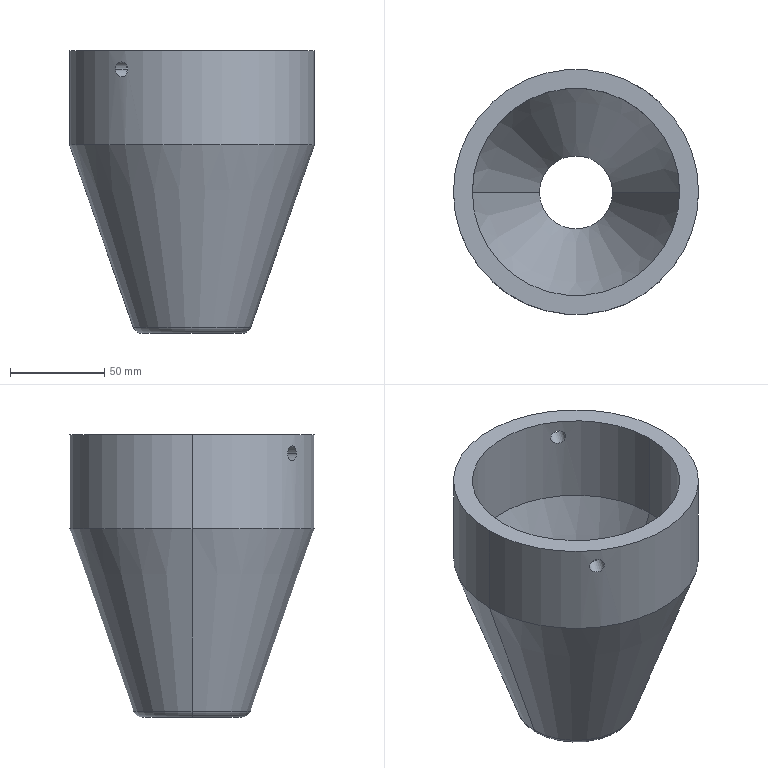Part | SolidWorks | features HoleWzd 2, 3DProfileFeature 1, Fillet 1, Revolution 1 | 1 solid | 16 faces | box 130 x 130 x 150 mm | volume 468175 mm3 | cylinder 8 | cone 4 | torus 2 | plane 2 | commonest cylinder face diameters 8 x4 110 x2 130 x2
STEP:
#1=CARTESIAN_POINT('',(552.403,234.744,-1661.65));
#2=VERTEX_POINT('',#1);
#3=CARTESIAN_POINT('',(490.059,234.744,-1661.65));
#4=VERTEX_POINT('',#3);
#5=CARTESIAN_POINT('',(521.231,234.744,-1661.65));
#6=DIRECTION('',(0.,0.,1.));
#7=DIRECTION('',(-1.,0.,0.));
#8=AXIS2_PLACEMENT_3D('',#5,#6,#7);
#9=CIRCLE('',#8,31.172);
#10=EDGE_CURVE('',#2,#4,#9,.T.);
#11=ORIENTED_EDGE('',*,*,#10,.F.);
#12=CARTESIAN_POINT('',(547.683,234.744,-1664.998));
#13=VERTEX_POINT('',#12);
#14=CARTESIAN_POINT('',(547.683,234.744,-1659.998));
#15=DIRECTION('',(0.,1.,0.));
#16=DIRECTION('',(-1.,0.,0.));
#17=AXIS2_PLACEMENT_3D('',#14,#15,#16);
#18=CIRCLE('',#17,5.);
#19=EDGE_CURVE('',#2,#13,#18,.T.);
#20=ORIENTED_EDGE('',*,*,#19,.T.);
#21=CARTESIAN_POINT('',(494.778,234.744,-1664.998));
#22=VERTEX_POINT('',#21);
#23=CARTESIAN_POINT('',(521.231,234.744,-1664.998));
#24=DIRECTION('',(0.,0.,-1.));
#25=DIRECTION('',(-1.,0.,0.));
#26=AXIS2_PLACEMENT_3D('',#23,#24,#25);
#27=CIRCLE('',#26,26.453);
#28=EDGE_CURVE('',#22,#13,#27,.T.);
#29=ORIENTED_EDGE('',*,*,#28,.F.);
#30=CARTESIAN_POINT('',(494.778,234.744,-1659.998));
#31=DIRECTION('',(0.,-1.,0.));
#32=DIRECTION('',(0.,0.,-1.));
#33=AXIS2_PLACEMENT_3D('',#30,#31,#32);
#34=CIRCLE('',#33,5.);
#35=EDGE_CURVE('',#4,#22,#34,.T.);
#36=ORIENTED_EDGE('',*,*,#35,.F.);
#37=EDGE_LOOP('',(#11,#20,#29,#36));
#38=FACE_OUTER_BOUND('',#37,.T.);
#39=CARTESIAN_POINT('',(521.231,234.744,-1659.998));
#40=DIRECTION('',(0.,0.,-1.));
#41=DIRECTION('',(-1.,0.,0.));
#42=AXIS2_PLACEMENT_3D('',#39,#40,#41);
#43=TOROIDAL_SURFACE('',#42,26.453,5.);
#44=ADVANCED_FACE('',(#38),#43,.T.);
#45=CARTESIAN_POINT('',(480.63,183.984,-1524.998));
#46=VERTEX_POINT('',#45);
#47=CARTESIAN_POINT('',(487.173,179.381,-1524.998));
#48=VERTEX_POINT('',#47);
#49=CARTESIAN_POINT('',(480.63,183.984,-1524.998));
#50=CARTESIAN_POINT('',(480.63,183.984,-1525.263));
#51=CARTESIAN_POINT('',(480.65,183.968,-1525.523));
#52=CARTESIAN_POINT('',(480.73,183.904,-1526.034));
#53=CARTESIAN_POINT('',(480.79,183.856,-1526.288));
#54=CARTESIAN_POINT('',(480.948,183.731,-1526.773));
#55=CARTESIAN_POINT('',(481.044,183.655,-1527.002));
#56=CARTESIAN_POINT('',(481.273,183.476,-1527.437));
#57=CARTESIAN_POINT('',(481.407,183.372,-1527.643));
#58=CARTESIAN_POINT('',(481.699,183.146,-1528.012));
#59=CARTESIAN_POINT('',(481.859,183.024,-1528.177));
#60=CARTESIAN_POINT('',(482.209,182.76,-1528.47));
#61=CARTESIAN_POINT('',(482.395,182.621,-1528.594));
#62=CARTESIAN_POINT('',(482.782,182.334,-1528.793));
#63=CARTESIAN_POINT('',(482.986,182.185,-1528.87));
#64=CARTESIAN_POINT('',(483.405,181.883,-1528.973));
#65=CARTESIAN_POINT('',(483.616,181.733,-1528.998));
#66=CARTESIAN_POINT('',(484.043,181.432,-1528.999));
#67=CARTESIAN_POINT('',(484.261,181.281,-1528.973));
#68=CARTESIAN_POINT('',(484.684,180.991,-1528.87));
#69=CARTESIAN_POINT('',(484.89,180.851,-1528.795));
#70=CARTESIAN_POINT('',(485.293,180.582,-1528.594));
#71=CARTESIAN_POINT('',(485.489,180.453,-1528.469));
#72=CARTESIAN_POINT('',(485.852,180.215,-1528.179));
#73=CARTESIAN_POINT('',(486.021,180.106,-1528.014));
#74=CARTESIAN_POINT('',(486.336,179.904,-1527.641));
#75=CARTESIAN_POINT('',(486.476,179.815,-1527.438));
#76=CARTESIAN_POINT('',(486.722,179.661,-1527.005));
#77=CARTESIAN_POINT('',(486.828,179.594,-1526.771));
#78=CARTESIAN_POINT('',(486.999,179.488,-1526.287));
#79=CARTESIAN_POINT('',(487.063,179.448,-1526.037));
#80=CARTESIAN_POINT('',(487.151,179.395,-1525.525));
#81=CARTESIAN_POINT('',(487.173,179.381,-1525.26));
#82=CARTESIAN_POINT('',(487.173,179.381,-1524.998));
#83=B_SPLINE_CURVE_WITH_KNOTS('',3,(#49,#50,#51,#52,#53,#54,#55,#56,#57,#58,#59,#60,#61,#62,#63,#64,#65,#66,#67,#68,#69,#70,#71,#72,#73,#74,#75,#76,#77,#78,#79,#80,#81,#82),.UNSPECIFIED.,.F.,.F.,(4,2,2,2,2,2,2,2,2,2,2,2,2,2,2,2,4),(0.,0.0007818,0.001564,0.002345,0.003127,0.003909,0.004691,0.005473,0.006254,0.007036,0.007818,0.0086,0.009382,0.01016,0.01095,0.01173,0.01251),.UNSPECIFIED.);
#84=EDGE_CURVE('',#46,#48,#83,.T.);
#85=ORIENTED_EDGE('',*,*,#84,.T.);
#86=CARTESIAN_POINT('',(492.94,187.578,-1524.998));
#87=VERTEX_POINT('',#86);
#88=CARTESIAN_POINT('',(561.902,285.605,-1524.998));
#89=DIRECTION('',(0.5754,0.8179,0.));
#90=VECTOR('',#89,1000.);
#91=LINE('',#88,#90);
#92=EDGE_CURVE('',#48,#87,#91,.T.);
#93=ORIENTED_EDGE('',*,*,#92,.T.);
#94=CARTESIAN_POINT('',(486.397,192.181,-1524.998));
#95=VERTEX_POINT('',#94);
#96=CARTESIAN_POINT('',(486.397,192.181,-1524.998));
#97=CARTESIAN_POINT('',(486.397,192.181,-1525.263));
#98=CARTESIAN_POINT('',(486.417,192.165,-1525.523));
#99=CARTESIAN_POINT('',(486.496,192.1,-1526.034));
#100=CARTESIAN_POINT('',(486.556,192.051,-1526.288));
#101=CARTESIAN_POINT('',(486.712,191.925,-1526.773));
#102=CARTESIAN_POINT('',(486.808,191.848,-1527.002));
#103=CARTESIAN_POINT('',(487.035,191.666,-1527.437));
#104=CARTESIAN_POINT('',(487.168,191.561,-1527.643));
#105=CARTESIAN_POINT('',(487.459,191.333,-1528.012));
#106=CARTESIAN_POINT('',(487.618,191.21,-1528.177));
#107=CARTESIAN_POINT('',(487.966,190.943,-1528.47));
#108=CARTESIAN_POINT('',(488.151,190.803,-1528.594));
#109=CARTESIAN_POINT('',(488.537,190.515,-1528.793));
#110=CARTESIAN_POINT('',(488.74,190.365,-1528.87));
#111=CARTESIAN_POINT('',(489.159,190.062,-1528.973));
#112=CARTESIAN_POINT('',(489.37,189.911,-1528.998));
#113=CARTESIAN_POINT('',(489.797,189.611,-1528.999));
#114=CARTESIAN_POINT('',(490.015,189.46,-1528.973));
#115=CARTESIAN_POINT('',(490.438,189.171,-1528.87));
#116=CARTESIAN_POINT('',(490.646,189.032,-1528.795));
#117=CARTESIAN_POINT('',(491.049,188.764,-1528.594));
#118=CARTESIAN_POINT('',(491.246,188.636,-1528.469));
#119=CARTESIAN_POINT('',(491.61,188.401,-1528.179));
#120=CARTESIAN_POINT('',(491.781,188.292,-1528.014));
#121=CARTESIAN_POINT('',(492.097,188.093,-1527.641));
#122=CARTESIAN_POINT('',(492.238,188.006,-1527.439));
#123=CARTESIAN_POINT('',(492.485,187.853,-1527.005));
#124=CARTESIAN_POINT('',(492.592,187.788,-1526.772));
#125=CARTESIAN_POINT('',(492.764,187.684,-1526.287));
#126=CARTESIAN_POINT('',(492.829,187.644,-1526.037));
#127=CARTESIAN_POINT('',(492.917,187.591,-1525.525));
#128=CARTESIAN_POINT('',(492.94,187.578,-1525.26));
#129=CARTESIAN_POINT('',(492.94,187.578,-1524.998));
#130=B_SPLINE_CURVE_WITH_KNOTS('',3,(#96,#97,#98,#99,#100,#101,#102,#103,#104,#105,#106,#107,#108,#109,#110,#111,#112,#113,#114,#115,#116,#117,#118,#119,#120,#121,#122,#123,#124,#125,#126,#127,#128,#129),.UNSPECIFIED.,.F.,.F.,(4,2,2,2,2,2,2,2,2,2,2,2,2,2,2,2,4),(0.,0.0007819,0.001564,0.002346,0.003127,0.003909,0.004691,0.005473,0.006255,0.007037,0.007819,0.008601,0.009382,0.01016,0.01095,0.01173,0.01251),.UNSPECIFIED.);
#131=EDGE_CURVE('',#95,#87,#130,.T.);
#132=ORIENTED_EDGE('',*,*,#131,.F.);
#133=CARTESIAN_POINT('',(555.359,290.208,-1524.998));
#134=DIRECTION('',(0.5754,0.8179,0.));
#135=VECTOR('',#134,1000.);
#136=LINE('',#133,#135);
#137=EDGE_CURVE('',#46,#95,#136,.T.);
#138=ORIENTED_EDGE('',*,*,#137,.F.);
#139=EDGE_LOOP('',(#85,#93,#132,#138));
#140=FACE_OUTER_BOUND('',#139,.T.);
#141=CARTESIAN_POINT('',(558.631,287.906,-1524.998));
#142=DIRECTION('',(0.5754,0.8179,0.));
#143=DIRECTION('',(-0.8179,0.5754,0.));
#144=AXIS2_PLACEMENT_3D('',#141,#142,#143);
#145=CYLINDRICAL_SURFACE('',#144,4.);
#146=ADVANCED_FACE('',(#140),#145,.F.);
#147=CARTESIAN_POINT('',(556.065,277.307,-1524.998));
#148=VERTEX_POINT('',#147);
#149=CARTESIAN_POINT('',(549.522,281.91,-1524.998));
#150=VERTEX_POINT('',#149);
#151=CARTESIAN_POINT('',(556.065,277.307,-1524.998));
#152=CARTESIAN_POINT('',(556.065,277.307,-1525.259));
#153=CARTESIAN_POINT('',(556.045,277.323,-1525.519));
#154=CARTESIAN_POINT('',(555.965,277.388,-1526.035));
#155=CARTESIAN_POINT('',(555.906,277.436,-1526.288));
#156=CARTESIAN_POINT('',(555.751,277.562,-1526.769));
#157=CARTESIAN_POINT('',(555.654,277.64,-1527.001));
#158=CARTESIAN_POINT('',(555.425,277.823,-1527.439));
#159=CARTESIAN_POINT('',(555.295,277.926,-1527.64));
#160=CARTESIAN_POINT('',(555.005,278.153,-1528.009));
#161=CARTESIAN_POINT('',(554.842,278.279,-1528.178));
#162=CARTESIAN_POINT('',(554.497,278.544,-1528.469));
#163=CARTESIAN_POINT('',(554.313,278.682,-1528.592));
#164=CARTESIAN_POINT('',(553.926,278.972,-1528.793));
#165=CARTESIAN_POINT('',(553.721,279.123,-1528.87));
#166=CARTESIAN_POINT('',(553.307,279.423,-1528.972));
#167=CARTESIAN_POINT('',(553.095,279.574,-1528.998));
#168=CARTESIAN_POINT('',(552.664,279.878,-1528.999));
#169=CARTESIAN_POINT('',(552.449,280.026,-1528.973));
#170=CARTESIAN_POINT('',(552.027,280.314,-1528.872));
#171=CARTESIAN_POINT('',(551.816,280.456,-1528.795));
#172=CARTESIAN_POINT('',(551.412,280.724,-1528.594));
#173=CARTESIAN_POINT('',(551.219,280.85,-1528.472));
#174=CARTESIAN_POINT('',(550.854,281.085,-1528.182));
#175=CARTESIAN_POINT('',(550.68,281.196,-1528.013));
#176=CARTESIAN_POINT('',(550.367,281.393,-1527.644));
#177=CARTESIAN_POINT('',(550.226,281.48,-1527.443));
#178=CARTESIAN_POINT('',(549.977,281.634,-1527.007));
#179=CARTESIAN_POINT('',(549.87,281.699,-1526.774));
#180=CARTESIAN_POINT('',(549.699,281.803,-1526.293));
#181=CARTESIAN_POINT('',(549.633,281.843,-1526.042));
#182=CARTESIAN_POINT('',(549.544,281.897,-1525.524));
#183=CARTESIAN_POINT('',(549.522,281.91,-1525.263));
#184=CARTESIAN_POINT('',(549.522,281.91,-1524.998));
#185=B_SPLINE_CURVE_WITH_KNOTS('',3,(#151,#152,#153,#154,#155,#156,#157,#158,#159,#160,#161,#162,#163,#164,#165,#166,#167,#168,#169,#170,#171,#172,#173,#174,#175,#176,#177,#178,#179,#180,#181,#182,#183,#184),.UNSPECIFIED.,.F.,.F.,(4,2,2,2,2,2,2,2,2,2,2,2,2,2,2,2,4),(0.01251,0.01329,0.01407,0.01486,0.01564,0.01642,0.0172,0.01798,0.01876,0.01955,0.02033,0.02111,0.02189,0.02267,0.02345,0.02424,0.02502),.UNSPECIFIED.);
#186=EDGE_CURVE('',#148,#150,#185,.T.);
#187=ORIENTED_EDGE('',*,*,#186,.F.);
#188=CARTESIAN_POINT('',(561.831,285.504,-1524.998));
#189=VERTEX_POINT('',#188);
#190=CARTESIAN_POINT('',(561.902,285.605,-1524.998));
#191=DIRECTION('',(0.5754,0.8179,0.));
#192=VECTOR('',#191,1000.);
#193=LINE('',#190,#192);
#194=EDGE_CURVE('',#148,#189,#193,.T.);
#195=ORIENTED_EDGE('',*,*,#194,.T.);
#196=CARTESIAN_POINT('',(555.288,290.107,-1524.998));
#197=VERTEX_POINT('',#196);
#198=CARTESIAN_POINT('',(561.831,285.504,-1524.998));
#199=CARTESIAN_POINT('',(561.831,285.504,-1525.259));
#200=CARTESIAN_POINT('',(561.812,285.52,-1525.519));
#201=CARTESIAN_POINT('',(561.731,285.584,-1526.035));
#202=CARTESIAN_POINT('',(561.671,285.632,-1526.287));
#203=CARTESIAN_POINT('',(561.515,285.756,-1526.769));
#204=CARTESIAN_POINT('',(561.418,285.832,-1527.001));
#205=CARTESIAN_POINT('',(561.187,286.013,-1527.439));
#206=CARTESIAN_POINT('',(561.056,286.115,-1527.64));
#207=CARTESIAN_POINT('',(560.764,286.34,-1528.009));
#208=CARTESIAN_POINT('',(560.601,286.465,-1528.178));
#209=CARTESIAN_POINT('',(560.254,286.727,-1528.469));
#210=CARTESIAN_POINT('',(560.07,286.865,-1528.592));
#211=CARTESIAN_POINT('',(559.681,287.153,-1528.793));
#212=CARTESIAN_POINT('',(559.475,287.303,-1528.87));
#213=CARTESIAN_POINT('',(559.061,287.602,-1528.972));
#214=CARTESIAN_POINT('',(558.849,287.753,-1528.998));
#215=CARTESIAN_POINT('',(558.418,288.056,-1528.999));
#216=CARTESIAN_POINT('',(558.203,288.205,-1528.973));
#217=CARTESIAN_POINT('',(557.782,288.494,-1528.872));
#218=CARTESIAN_POINT('',(557.572,288.636,-1528.795));
#219=CARTESIAN_POINT('',(557.168,288.906,-1528.594));
#220=CARTESIAN_POINT('',(556.977,289.033,-1528.472));
#221=CARTESIAN_POINT('',(556.612,289.271,-1528.182));
#222=CARTESIAN_POINT('',(556.439,289.383,-1528.013));
#223=CARTESIAN_POINT('',(556.128,289.582,-1527.644));
#224=CARTESIAN_POINT('',(555.988,289.671,-1527.443));
#225=CARTESIAN_POINT('',(555.74,289.827,-1527.007));
#226=CARTESIAN_POINT('',(555.634,289.893,-1526.774));
#227=CARTESIAN_POINT('',(555.464,289.999,-1526.293));
#228=CARTESIAN_POINT('',(555.399,290.039,-1526.042));
#229=CARTESIAN_POINT('',(555.31,290.093,-1525.524));
#230=CARTESIAN_POINT('',(555.288,290.107,-1525.263));
#231=CARTESIAN_POINT('',(555.288,290.107,-1524.998));
#232=B_SPLINE_CURVE_WITH_KNOTS('',3,(#198,#199,#200,#201,#202,#203,#204,#205,#206,#207,#208,#209,#210,#211,#212,#213,#214,#215,#216,#217,#218,#219,#220,#221,#222,#223,#224,#225,#226,#227,#228,#229,#230,#231),.UNSPECIFIED.,.F.,.F.,(4,2,2,2,2,2,2,2,2,2,2,2,2,2,2,2,4),(0.01251,0.01329,0.01407,0.01485,0.01564,0.01642,0.0172,0.01798,0.01876,0.01954,0.02032,0.02111,0.02189,0.02267,0.02345,0.02423,0.02501),.UNSPECIFIED.);
#233=EDGE_CURVE('',#189,#197,#232,.T.);
#234=ORIENTED_EDGE('',*,*,#233,.T.);
#235=CARTESIAN_POINT('',(555.359,290.208,-1524.998));
#236=DIRECTION('',(0.5754,0.8179,0.));
#237=VECTOR('',#236,1000.);
#238=LINE('',#235,#237);
#239=EDGE_CURVE('',#150,#197,#238,.T.);
#240=ORIENTED_EDGE('',*,*,#239,.F.);
#241=EDGE_LOOP('',(#187,#195,#234,#240));
#242=FACE_OUTER_BOUND('',#241,.T.);
#243=CARTESIAN_POINT('',(558.631,287.906,-1524.998));
#244=DIRECTION('',(0.5754,0.8179,0.));
#245=DIRECTION('',(-0.8179,0.5754,0.));
#246=AXIS2_PLACEMENT_3D('',#243,#244,#245);
#247=CYLINDRICAL_SURFACE('',#246,4.);
#248=ADVANCED_FACE('',(#242),#247,.F.);
#249=ORIENTED_EDGE('',*,*,#131,.T.);
#250=CARTESIAN_POINT('',(492.94,187.578,-1524.998));
#251=CARTESIAN_POINT('',(492.94,187.578,-1524.737));
#252=CARTESIAN_POINT('',(492.918,187.591,-1524.478));
#253=CARTESIAN_POINT('',(492.83,187.644,-1523.962));
#254=CARTESIAN_POINT('',(492.764,187.684,-1523.709));
#255=CARTESIAN_POINT('',(492.593,187.787,-1523.228));
#256=CARTESIAN_POINT('',(492.488,187.852,-1522.996));
#257=CARTESIAN_POINT('',(492.238,188.006,-1522.558));
#258=CARTESIAN_POINT('',(492.097,188.093,-1522.356));
#259=CARTESIAN_POINT('',(491.785,188.29,-1521.987));
#260=CARTESIAN_POINT('',(491.611,188.4,-1521.819));
#261=CARTESIAN_POINT('',(491.246,188.636,-1521.528));
#262=CARTESIAN_POINT('',(491.053,188.761,-1521.405));
#263=CARTESIAN_POINT('',(490.65,189.029,-1521.204));
#264=CARTESIAN_POINT('',(490.439,189.171,-1521.127));
#265=CARTESIAN_POINT('',(490.017,189.459,-1521.025));
#266=CARTESIAN_POINT('',(489.803,189.607,-1520.999));
#267=CARTESIAN_POINT('',(489.371,189.91,-1520.998));
#268=CARTESIAN_POINT('',(489.159,190.062,-1521.024));
#269=CARTESIAN_POINT('',(488.745,190.362,-1521.125));
#270=CARTESIAN_POINT('',(488.541,190.513,-1521.202));
#271=CARTESIAN_POINT('',(488.152,190.803,-1521.402));
#272=CARTESIAN_POINT('',(487.968,190.941,-1521.525));
#273=CARTESIAN_POINT('',(487.623,191.206,-1521.815));
#274=CARTESIAN_POINT('',(487.46,191.332,-1521.984));
#275=CARTESIAN_POINT('',(487.169,191.56,-1522.352));
#276=CARTESIAN_POINT('',(487.039,191.663,-1522.554));
#277=CARTESIAN_POINT('',(486.81,191.846,-1522.99));
#278=CARTESIAN_POINT('',(486.713,191.924,-1523.223));
#279=CARTESIAN_POINT('',(486.557,192.05,-1523.704));
#280=CARTESIAN_POINT('',(486.497,192.099,-1523.955));
#281=CARTESIAN_POINT('',(486.417,192.165,-1524.473));
#282=CARTESIAN_POINT('',(486.397,192.181,-1524.734));
#283=CARTESIAN_POINT('',(486.397,192.181,-1524.998));
#284=B_SPLINE_CURVE_WITH_KNOTS('',3,(#250,#251,#252,#253,#254,#255,#256,#257,#258,#259,#260,#261,#262,#263,#264,#265,#266,#267,#268,#269,#270,#271,#272,#273,#274,#275,#276,#277,#278,#279,#280,#281,#282,#283),.UNSPECIFIED.,.F.,.F.,(4,2,2,2,2,2,2,2,2,2,2,2,2,2,2,2,4),(0.01251,0.01329,0.01407,0.01486,0.01564,0.01642,0.0172,0.01798,0.01876,0.01955,0.02033,0.02111,0.02189,0.02267,0.02345,0.02424,0.02502),.UNSPECIFIED.);
#285=EDGE_CURVE('',#87,#95,#284,.T.);
#286=ORIENTED_EDGE('',*,*,#285,.T.);
#287=EDGE_LOOP('',(#249,#286));
#288=FACE_BOUND('',#287,.T.);
#289=CARTESIAN_POINT('',(466.231,234.744,-1563.299));
#290=VERTEX_POINT('',#289);
#291=CARTESIAN_POINT('',(576.231,234.744,-1563.299));
#292=VERTEX_POINT('',#291);
#293=CARTESIAN_POINT('',(521.231,234.744,-1563.299));
#294=DIRECTION('',(0.,0.,1.));
#295=DIRECTION('',(1.,0.,0.));
#296=AXIS2_PLACEMENT_3D('',#293,#294,#295);
#297=CIRCLE('',#296,55.);
#298=EDGE_CURVE('',#290,#292,#297,.T.);
#299=ORIENTED_EDGE('',*,*,#298,.F.);
#300=CARTESIAN_POINT('',(466.231,234.744,-1514.998));
#301=VERTEX_POINT('',#300);
#302=CARTESIAN_POINT('',(466.231,234.744,-1514.998));
#303=DIRECTION('',(0.,0.,1.));
#304=VECTOR('',#303,1000.);
#305=LINE('',#302,#304);
#306=EDGE_CURVE('',#290,#301,#305,.T.);
#307=ORIENTED_EDGE('',*,*,#306,.T.);
#308=CARTESIAN_POINT('',(576.231,234.744,-1514.998));
#309=VERTEX_POINT('',#308);
#310=CARTESIAN_POINT('',(521.231,234.744,-1514.998));
#311=DIRECTION('',(0.,0.,1.));
#312=DIRECTION('',(1.,0.,0.));
#313=AXIS2_PLACEMENT_3D('',#310,#311,#312);
#314=CIRCLE('',#313,55.);
#315=EDGE_CURVE('',#301,#309,#314,.T.);
#316=ORIENTED_EDGE('',*,*,#315,.T.);
#317=CARTESIAN_POINT('',(576.231,234.744,-1514.998));
#318=DIRECTION('',(0.,0.,1.));
#319=VECTOR('',#318,1000.);
#320=LINE('',#317,#319);
#321=EDGE_CURVE('',#292,#309,#320,.T.);
#322=ORIENTED_EDGE('',*,*,#321,.F.);
#323=EDGE_LOOP('',(#299,#307,#316,#322));
#324=FACE_OUTER_BOUND('',#323,.T.);
#325=CARTESIAN_POINT('',(521.231,234.744,-1514.998));
#326=DIRECTION('',(0.,0.,1.));
#327=DIRECTION('',(1.,0.,0.));
#328=AXIS2_PLACEMENT_3D('',#325,#326,#327);
#329=CYLINDRICAL_SURFACE('',#328,55.);
#330=ADVANCED_FACE('',(#288,#324),#329,.F.);
#331=CARTESIAN_POINT('',(540.636,234.744,-1664.998));
#332=VERTEX_POINT('',#331);
#333=CARTESIAN_POINT('',(501.825,234.744,-1664.998));
#334=VERTEX_POINT('',#333);
#335=CARTESIAN_POINT('',(521.231,234.744,-1664.998));
#336=DIRECTION('',(0.,0.,-1.));
#337=DIRECTION('',(-1.,0.,0.));
#338=AXIS2_PLACEMENT_3D('',#335,#336,#337);
#339=CIRCLE('',#338,19.405);
#340=EDGE_CURVE('',#332,#334,#339,.T.);
#341=ORIENTED_EDGE('',*,*,#340,.T.);
#342=CARTESIAN_POINT('',(466.231,234.744,-1563.299));
#343=DIRECTION('',(-0.3304,0.,0.9439));
#344=VECTOR('',#343,1000.);
#345=LINE('',#342,#344);
#346=EDGE_CURVE('',#334,#290,#345,.T.);
#347=ORIENTED_EDGE('',*,*,#346,.T.);
#348=ORIENTED_EDGE('',*,*,#298,.T.);
#349=CARTESIAN_POINT('',(576.231,234.744,-1563.299));
#350=DIRECTION('',(0.3304,0.,0.9439));
#351=VECTOR('',#350,1000.);
#352=LINE('',#349,#351);
#353=EDGE_CURVE('',#332,#292,#352,.T.);
#354=ORIENTED_EDGE('',*,*,#353,.F.);
#355=EDGE_LOOP('',(#341,#347,#348,#354));
#356=FACE_OUTER_BOUND('',#355,.T.);
#357=CARTESIAN_POINT('',(521.231,234.744,-1563.299));
#358=DIRECTION('',(0.,0.,1.));
#359=DIRECTION('',(1.,0.,0.));
#360=AXIS2_PLACEMENT_3D('',#357,#358,#359);
#361=CONICAL_SURFACE('',#360,55.,0.3367);
#362=ADVANCED_FACE('',(#356),#361,.F.);
#363=CARTESIAN_POINT('',(555.288,290.107,-1524.998));
#364=CARTESIAN_POINT('',(555.288,290.107,-1524.734));
#365=CARTESIAN_POINT('',(555.31,290.093,-1524.474));
#366=CARTESIAN_POINT('',(555.397,290.04,-1523.963));
#367=CARTESIAN_POINT('',(555.463,290.,-1523.709));
#368=CARTESIAN_POINT('',(555.634,289.893,-1523.224));
#369=CARTESIAN_POINT('',(555.738,289.828,-1522.995));
#370=CARTESIAN_POINT('',(555.984,289.673,-1522.56));
#371=CARTESIAN_POINT('',(556.127,289.583,-1522.354));
#372=CARTESIAN_POINT('',(556.438,289.384,-1521.985));
#373=CARTESIAN_POINT('',(556.607,289.274,-1521.819));
#374=CARTESIAN_POINT('',(556.974,289.035,-1521.527));
#375=CARTESIAN_POINT('',(557.168,288.906,-1521.403));
#376=CARTESIAN_POINT('',(557.568,288.639,-1521.203));
#377=CARTESIAN_POINT('',(557.777,288.497,-1521.127));
#378=CARTESIAN_POINT('',(558.203,288.205,-1521.024));
#379=CARTESIAN_POINT('',(558.416,288.057,-1520.999));
#380=CARTESIAN_POINT('',(558.843,287.757,-1520.998));
#381=CARTESIAN_POINT('',(559.059,287.603,-1521.024));
#382=CARTESIAN_POINT('',(559.475,287.303,-1521.127));
#383=CARTESIAN_POINT('',(559.676,287.156,-1521.202));
#384=CARTESIAN_POINT('',(560.066,286.868,-1521.403));
#385=CARTESIAN_POINT('',(560.253,286.727,-1521.528));
#386=CARTESIAN_POINT('',(560.599,286.466,-1521.817));
#387=CARTESIAN_POINT('',(560.76,286.343,-1521.983));
#388=CARTESIAN_POINT('',(561.056,286.115,-1522.356));
#389=CARTESIAN_POINT('',(561.187,286.013,-1522.558));
#390=CARTESIAN_POINT('',(561.415,285.834,-1522.992));
#391=CARTESIAN_POINT('',(561.514,285.756,-1523.225));
#392=CARTESIAN_POINT('',(561.672,285.632,-1523.71));
#393=CARTESIAN_POINT('',(561.731,285.584,-1523.96));
#394=CARTESIAN_POINT('',(561.811,285.52,-1524.472));
#395=CARTESIAN_POINT('',(561.831,285.504,-1524.737));
#396=CARTESIAN_POINT('',(561.831,285.504,-1524.998));
#397=B_SPLINE_CURVE_WITH_KNOTS('',3,(#363,#364,#365,#366,#367,#368,#369,#370,#371,#372,#373,#374,#375,#376,#377,#378,#379,#380,#381,#382,#383,#384,#385,#386,#387,#388,#389,#390,#391,#392,#393,#394,#395,#396),.UNSPECIFIED.,.F.,.F.,(4,2,2,2,2,2,2,2,2,2,2,2,2,2,2,2,4),(0.,0.0007818,0.001564,0.002345,0.003127,0.003909,0.004691,0.005473,0.006254,0.007036,0.007818,0.0086,0.009382,0.01016,0.01095,0.01173,0.01251),.UNSPECIFIED.);
#398=EDGE_CURVE('',#197,#189,#397,.T.);
#399=ORIENTED_EDGE('',*,*,#398,.F.);
#400=ORIENTED_EDGE('',*,*,#233,.F.);
#401=EDGE_LOOP('',(#399,#400));
#402=FACE_BOUND('',#401,.T.);
#403=CARTESIAN_POINT('',(586.231,234.744,-1564.998));
#404=VERTEX_POINT('',#403);
#405=CARTESIAN_POINT('',(456.231,234.744,-1564.998));
#406=VERTEX_POINT('',#405);
#407=CARTESIAN_POINT('',(521.231,234.744,-1564.998));
#408=DIRECTION('',(0.,0.,1.));
#409=DIRECTION('',(1.,0.,0.));
#410=AXIS2_PLACEMENT_3D('',#407,#408,#409);
#411=CIRCLE('',#410,65.);
#412=EDGE_CURVE('',#404,#406,#411,.T.);
#413=ORIENTED_EDGE('',*,*,#412,.T.);
#414=CARTESIAN_POINT('',(456.231,234.744,-1514.998));
#415=VERTEX_POINT('',#414);
#416=CARTESIAN_POINT('',(456.231,234.744,-1664.998));
#417=DIRECTION('',(0.,0.,1.));
#418=VECTOR('',#417,1000.);
#419=LINE('',#416,#418);
#420=EDGE_CURVE('',#406,#415,#419,.T.);
#421=ORIENTED_EDGE('',*,*,#420,.T.);
#422=CARTESIAN_POINT('',(586.231,234.744,-1514.998));
#423=VERTEX_POINT('',#422);
#424=CARTESIAN_POINT('',(521.231,234.744,-1514.998));
#425=DIRECTION('',(0.,0.,1.));
#426=DIRECTION('',(1.,0.,0.));
#427=AXIS2_PLACEMENT_3D('',#424,#425,#426);
#428=CIRCLE('',#427,65.);
#429=EDGE_CURVE('',#423,#415,#428,.T.);
#430=ORIENTED_EDGE('',*,*,#429,.F.);
#431=CARTESIAN_POINT('',(586.231,234.744,-1664.998));
#432=DIRECTION('',(0.,0.,1.));
#433=VECTOR('',#432,1000.);
#434=LINE('',#431,#433);
#435=EDGE_CURVE('',#404,#423,#434,.T.);
#436=ORIENTED_EDGE('',*,*,#435,.F.);
#437=EDGE_LOOP('',(#413,#421,#430,#436));
#438=FACE_OUTER_BOUND('',#437,.T.);
#439=CARTESIAN_POINT('',(521.231,234.744,-1664.998));
#440=DIRECTION('',(0.,0.,1.));
#441=DIRECTION('',(1.,0.,0.));
#442=AXIS2_PLACEMENT_3D('',#439,#440,#441);
#443=CYLINDRICAL_SURFACE('',#442,65.);
#444=ADVANCED_FACE('',(#402,#438),#443,.T.);
#445=ORIENTED_EDGE('',*,*,#10,.T.);
#446=CARTESIAN_POINT('',(456.231,234.744,-1564.998));
#447=DIRECTION('',(-0.3304,0.,0.9439));
#448=VECTOR('',#447,1000.);
#449=LINE('',#446,#448);
#450=EDGE_CURVE('',#4,#406,#449,.T.);
#451=ORIENTED_EDGE('',*,*,#450,.T.);
#452=ORIENTED_EDGE('',*,*,#412,.F.);
#453=CARTESIAN_POINT('',(586.231,234.744,-1564.998));
#454=DIRECTION('',(0.3304,0.,0.9439));
#455=VECTOR('',#454,1000.);
#456=LINE('',#453,#455);
#457=EDGE_CURVE('',#2,#404,#456,.T.);
#458=ORIENTED_EDGE('',*,*,#457,.F.);
#459=EDGE_LOOP('',(#445,#451,#452,#458));
#460=FACE_OUTER_BOUND('',#459,.T.);
#461=CARTESIAN_POINT('',(521.231,234.744,-1564.998));
#462=DIRECTION('',(0.,0.,1.));
#463=DIRECTION('',(1.,0.,0.));
#464=AXIS2_PLACEMENT_3D('',#461,#462,#463);
#465=CONICAL_SURFACE('',#464,65.,0.3367);
#466=ADVANCED_FACE('',(#460),#465,.T.);
#467=ORIENTED_EDGE('',*,*,#450,.F.);
#468=CARTESIAN_POINT('',(521.231,234.744,-1661.65));
#469=DIRECTION('',(0.,0.,1.));
#470=DIRECTION('',(-1.,0.,0.));
#471=AXIS2_PLACEMENT_3D('',#468,#469,#470);
#472=CIRCLE('',#471,31.172);
#473=EDGE_CURVE('',#4,#2,#472,.T.);
#474=ORIENTED_EDGE('',*,*,#473,.T.);
#475=ORIENTED_EDGE('',*,*,#457,.T.);
#476=CARTESIAN_POINT('',(521.231,234.744,-1564.998));
#477=DIRECTION('',(0.,0.,1.));
#478=DIRECTION('',(1.,0.,0.));
#479=AXIS2_PLACEMENT_3D('',#476,#477,#478);
#480=CIRCLE('',#479,65.);
#481=EDGE_CURVE('',#406,#404,#480,.T.);
#482=ORIENTED_EDGE('',*,*,#481,.F.);
#483=EDGE_LOOP('',(#467,#474,#475,#482));
#484=FACE_OUTER_BOUND('',#483,.T.);
#485=CARTESIAN_POINT('',(521.231,234.744,-1564.998));
#486=DIRECTION('',(0.,0.,1.));
#487=DIRECTION('',(1.,0.,0.));
#488=AXIS2_PLACEMENT_3D('',#485,#486,#487);
#489=CONICAL_SURFACE('',#488,65.,0.3367);
#490=ADVANCED_FACE('',(#484),#489,.T.);
#491=ORIENTED_EDGE('',*,*,#28,.T.);
#492=CARTESIAN_POINT('',(521.231,234.744,-1664.998));
#493=DIRECTION('',(0.,0.,-1.));
#494=DIRECTION('',(-1.,0.,0.));
#495=AXIS2_PLACEMENT_3D('',#492,#493,#494);
#496=CIRCLE('',#495,26.453);
#497=EDGE_CURVE('',#13,#22,#496,.T.);
#498=ORIENTED_EDGE('',*,*,#497,.T.);
#499=EDGE_LOOP('',(#491,#498));
#500=FACE_OUTER_BOUND('',#499,.T.);
#501=ORIENTED_EDGE('',*,*,#340,.F.);
#502=CARTESIAN_POINT('',(521.231,234.744,-1664.998));
#503=DIRECTION('',(0.,0.,-1.));
#504=DIRECTION('',(-1.,0.,0.));
#505=AXIS2_PLACEMENT_3D('',#502,#503,#504);
#506=CIRCLE('',#505,19.405);
#507=EDGE_CURVE('',#334,#332,#506,.T.);
#508=ORIENTED_EDGE('',*,*,#507,.F.);
#509=EDGE_LOOP('',(#501,#508));
#510=FACE_BOUND('',#509,.T.);
#511=CARTESIAN_POINT('',(551.231,234.744,-1664.998));
#512=DIRECTION('',(0.,0.,-1.));
#513=DIRECTION('',(-1.,0.,0.));
#514=AXIS2_PLACEMENT_3D('',#511,#512,#513);
#515=PLANE('',#514);
#516=ADVANCED_FACE('',(#500,#510),#515,.T.);
#517=CARTESIAN_POINT('',(521.231,234.744,-1514.998));
#518=DIRECTION('',(0.,0.,1.));
#519=DIRECTION('',(1.,0.,0.));
#520=AXIS2_PLACEMENT_3D('',#517,#518,#519);
#521=CIRCLE('',#520,55.);
#522=EDGE_CURVE('',#309,#301,#521,.T.);
#523=ORIENTED_EDGE('',*,*,#522,.F.);
#524=ORIENTED_EDGE('',*,*,#315,.F.);
#525=EDGE_LOOP('',(#523,#524));
#526=FACE_BOUND('',#525,.T.);
#527=ORIENTED_EDGE('',*,*,#429,.T.);
#528=CARTESIAN_POINT('',(521.231,234.744,-1514.998));
#529=DIRECTION('',(0.,0.,1.));
#530=DIRECTION('',(1.,0.,0.));
#531=AXIS2_PLACEMENT_3D('',#528,#529,#530);
#532=CIRCLE('',#531,65.);
#533=EDGE_CURVE('',#415,#423,#532,.T.);
#534=ORIENTED_EDGE('',*,*,#533,.T.);
#535=EDGE_LOOP('',(#527,#534));
#536=FACE_OUTER_BOUND('',#535,.T.);
#537=CARTESIAN_POINT('',(521.231,234.744,-1514.998));
#538=DIRECTION('',(0.,0.,1.));
#539=DIRECTION('',(1.,0.,0.));
#540=AXIS2_PLACEMENT_3D('',#537,#538,#539);
#541=PLANE('',#540);
#542=ADVANCED_FACE('',(#526,#536),#541,.T.);
#543=ORIENTED_EDGE('',*,*,#420,.F.);
#544=ORIENTED_EDGE('',*,*,#481,.T.);
#545=ORIENTED_EDGE('',*,*,#435,.T.);
#546=ORIENTED_EDGE('',*,*,#533,.F.);
#547=EDGE_LOOP('',(#543,#544,#545,#546));
#548=FACE_OUTER_BOUND('',#547,.T.);
#549=ORIENTED_EDGE('',*,*,#84,.F.);
#550=CARTESIAN_POINT('',(487.173,179.381,-1524.998));
#551=CARTESIAN_POINT('',(487.173,179.381,-1524.737));
#552=CARTESIAN_POINT('',(487.151,179.394,-1524.478));
#553=CARTESIAN_POINT('',(487.064,179.448,-1523.962));
#554=CARTESIAN_POINT('',(486.999,179.488,-1523.709));
#555=CARTESIAN_POINT('',(486.829,179.594,-1523.228));
#556=CARTESIAN_POINT('',(486.724,179.659,-1522.996));
#557=CARTESIAN_POINT('',(486.476,179.815,-1522.558));
#558=CARTESIAN_POINT('',(486.336,179.904,-1522.356));
#559=CARTESIAN_POINT('',(486.026,180.103,-1521.987));
#560=CARTESIAN_POINT('',(485.853,180.215,-1521.819));
#561=CARTESIAN_POINT('',(485.489,180.453,-1521.528));
#562=CARTESIAN_POINT('',(485.297,180.579,-1521.405));
#563=CARTESIAN_POINT('',(484.895,180.848,-1521.204));
#564=CARTESIAN_POINT('',(484.684,180.991,-1521.127));
#565=CARTESIAN_POINT('',(484.262,181.28,-1521.025));
#566=CARTESIAN_POINT('',(484.049,181.428,-1520.999));
#567=CARTESIAN_POINT('',(483.617,181.732,-1520.998));
#568=CARTESIAN_POINT('',(483.405,181.883,-1521.024));
#569=CARTESIAN_POINT('',(482.99,182.182,-1521.125));
#570=CARTESIAN_POINT('',(482.786,182.332,-1521.202));
#571=CARTESIAN_POINT('',(482.395,182.62,-1521.402));
#572=CARTESIAN_POINT('',(482.211,182.758,-1521.525));
#573=CARTESIAN_POINT('',(481.864,183.02,-1521.815));
#574=CARTESIAN_POINT('',(481.701,183.145,-1521.984));
#575=CARTESIAN_POINT('',(481.408,183.371,-1522.352));
#576=CARTESIAN_POINT('',(481.277,183.473,-1522.554));
#577=CARTESIAN_POINT('',(481.046,183.653,-1522.99));
#578=CARTESIAN_POINT('',(480.948,183.731,-1523.223));
#579=CARTESIAN_POINT('',(480.791,183.855,-1523.704));
#580=CARTESIAN_POINT('',(480.731,183.903,-1523.955));
#581=CARTESIAN_POINT('',(480.65,183.968,-1524.473));
#582=CARTESIAN_POINT('',(480.63,183.984,-1524.734));
#583=CARTESIAN_POINT('',(480.63,183.984,-1524.998));
#584=B_SPLINE_CURVE_WITH_KNOTS('',3,(#550,#551,#552,#553,#554,#555,#556,#557,#558,#559,#560,#561,#562,#563,#564,#565,#566,#567,#568,#569,#570,#571,#572,#573,#574,#575,#576,#577,#578,#579,#580,#581,#582,#583),.UNSPECIFIED.,.F.,.F.,(4,2,2,2,2,2,2,2,2,2,2,2,2,2,2,2,4),(0.01251,0.01329,0.01407,0.01485,0.01564,0.01642,0.0172,0.01798,0.01876,0.01954,0.02032,0.02111,0.02189,0.02267,0.02345,0.02423,0.02501),.UNSPECIFIED.);
#585=EDGE_CURVE('',#48,#46,#584,.T.);
#586=ORIENTED_EDGE('',*,*,#585,.F.);
#587=EDGE_LOOP('',(#549,#586));
#588=FACE_BOUND('',#587,.T.);
#589=CARTESIAN_POINT('',(521.231,234.744,-1664.998));
#590=DIRECTION('',(0.,0.,1.));
#591=DIRECTION('',(1.,0.,0.));
#592=AXIS2_PLACEMENT_3D('',#589,#590,#591);
#593=CYLINDRICAL_SURFACE('',#592,65.);
#594=ADVANCED_FACE('',(#548,#588),#593,.T.);
#595=ORIENTED_EDGE('',*,*,#346,.F.);
#596=ORIENTED_EDGE('',*,*,#507,.T.);
#597=ORIENTED_EDGE('',*,*,#353,.T.);
#598=CARTESIAN_POINT('',(521.231,234.744,-1563.299));
#599=DIRECTION('',(0.,0.,1.));
#600=DIRECTION('',(1.,0.,0.));
#601=AXIS2_PLACEMENT_3D('',#598,#599,#600);
#602=CIRCLE('',#601,55.);
#603=EDGE_CURVE('',#292,#290,#602,.T.);
#604=ORIENTED_EDGE('',*,*,#603,.T.);
#605=EDGE_LOOP('',(#595,#596,#597,#604));
#606=FACE_OUTER_BOUND('',#605,.T.);
#607=CARTESIAN_POINT('',(521.231,234.744,-1563.299));
#608=DIRECTION('',(0.,0.,1.));
#609=DIRECTION('',(1.,0.,0.));
#610=AXIS2_PLACEMENT_3D('',#607,#608,#609);
#611=CONICAL_SURFACE('',#610,55.,0.3367);
#612=ADVANCED_FACE('',(#606),#611,.F.);
#613=ORIENTED_EDGE('',*,*,#306,.F.);
#614=ORIENTED_EDGE('',*,*,#603,.F.);
#615=ORIENTED_EDGE('',*,*,#321,.T.);
#616=ORIENTED_EDGE('',*,*,#522,.T.);
#617=EDGE_LOOP('',(#613,#614,#615,#616));
#618=FACE_OUTER_BOUND('',#617,.T.);
#619=CARTESIAN_POINT('',(549.522,281.91,-1524.998));
#620=CARTESIAN_POINT('',(549.522,281.91,-1524.734));
#621=CARTESIAN_POINT('',(549.544,281.897,-1524.474));
#622=CARTESIAN_POINT('',(549.631,281.844,-1523.963));
#623=CARTESIAN_POINT('',(549.697,281.804,-1523.709));
#624=CARTESIAN_POINT('',(549.869,281.7,-1523.224));
#625=CARTESIAN_POINT('',(549.974,281.635,-1522.994));
#626=CARTESIAN_POINT('',(550.222,281.483,-1522.56));
#627=CARTESIAN_POINT('',(550.366,281.394,-1522.354));
#628=CARTESIAN_POINT('',(550.678,281.197,-1521.985));
#629=CARTESIAN_POINT('',(550.849,281.089,-1521.82));
#630=CARTESIAN_POINT('',(551.216,280.851,-1521.527));
#631=CARTESIAN_POINT('',(551.411,280.724,-1521.403));
#632=CARTESIAN_POINT('',(551.813,280.458,-1521.203));
#633=CARTESIAN_POINT('',(552.022,280.317,-1521.127));
#634=CARTESIAN_POINT('',(552.449,280.026,-1521.024));
#635=CARTESIAN_POINT('',(552.662,279.878,-1520.999));
#636=CARTESIAN_POINT('',(553.089,279.578,-1520.998));
#637=CARTESIAN_POINT('',(553.305,279.424,-1521.024));
#638=CARTESIAN_POINT('',(553.72,279.123,-1521.127));
#639=CARTESIAN_POINT('',(553.921,278.975,-1521.202));
#640=CARTESIAN_POINT('',(554.31,278.685,-1521.403));
#641=CARTESIAN_POINT('',(554.496,278.544,-1521.528));
#642=CARTESIAN_POINT('',(554.841,278.28,-1521.817));
#643=CARTESIAN_POINT('',(555.001,278.156,-1521.983));
#644=CARTESIAN_POINT('',(555.295,277.926,-1522.356));
#645=CARTESIAN_POINT('',(555.425,277.823,-1522.558));
#646=CARTESIAN_POINT('',(555.652,277.642,-1522.992));
#647=CARTESIAN_POINT('',(555.75,277.563,-1523.225));
#648=CARTESIAN_POINT('',(555.906,277.436,-1523.71));
#649=CARTESIAN_POINT('',(555.965,277.388,-1523.959));
#650=CARTESIAN_POINT('',(556.044,277.323,-1524.472));
#651=CARTESIAN_POINT('',(556.065,277.307,-1524.737));
#652=CARTESIAN_POINT('',(556.065,277.307,-1524.998));
#653=B_SPLINE_CURVE_WITH_KNOTS('',3,(#619,#620,#621,#622,#623,#624,#625,#626,#627,#628,#629,#630,#631,#632,#633,#634,#635,#636,#637,#638,#639,#640,#641,#642,#643,#644,#645,#646,#647,#648,#649,#650,#651,#652),.UNSPECIFIED.,.F.,.F.,(4,2,2,2,2,2,2,2,2,2,2,2,2,2,2,2,4),(0.,0.0007819,0.001564,0.002346,0.003127,0.003909,0.004691,0.005473,0.006255,0.007037,0.007819,0.008601,0.009382,0.01016,0.01095,0.01173,0.01251),.UNSPECIFIED.);
#654=EDGE_CURVE('',#150,#148,#653,.T.);
#655=ORIENTED_EDGE('',*,*,#654,.T.);
#656=ORIENTED_EDGE('',*,*,#186,.T.);
#657=EDGE_LOOP('',(#655,#656));
#658=FACE_BOUND('',#657,.T.);
#659=CARTESIAN_POINT('',(521.231,234.744,-1514.998));
#660=DIRECTION('',(0.,0.,1.));
#661=DIRECTION('',(1.,0.,0.));
#662=AXIS2_PLACEMENT_3D('',#659,#660,#661);
#663=CYLINDRICAL_SURFACE('',#662,55.);
#664=ADVANCED_FACE('',(#618,#658),#663,.F.);
#665=ORIENTED_EDGE('',*,*,#194,.F.);
#666=ORIENTED_EDGE('',*,*,#654,.F.);
#667=ORIENTED_EDGE('',*,*,#239,.T.);
#668=ORIENTED_EDGE('',*,*,#398,.T.);
#669=EDGE_LOOP('',(#665,#666,#667,#668));
#670=FACE_OUTER_BOUND('',#669,.T.);
#671=CARTESIAN_POINT('',(558.631,287.906,-1524.998));
#672=DIRECTION('',(0.5754,0.8179,0.));
#673=DIRECTION('',(-0.8179,0.5754,0.));
#674=AXIS2_PLACEMENT_3D('',#671,#672,#673);
#675=CYLINDRICAL_SURFACE('',#674,4.);
#676=ADVANCED_FACE('',(#670),#675,.F.);
#677=ORIENTED_EDGE('',*,*,#92,.F.);
#678=ORIENTED_EDGE('',*,*,#585,.T.);
#679=ORIENTED_EDGE('',*,*,#137,.T.);
#680=ORIENTED_EDGE('',*,*,#285,.F.);
#681=EDGE_LOOP('',(#677,#678,#679,#680));
#682=FACE_OUTER_BOUND('',#681,.T.);
#683=CARTESIAN_POINT('',(558.631,287.906,-1524.998));
#684=DIRECTION('',(0.5754,0.8179,0.));
#685=DIRECTION('',(-0.8179,0.5754,0.));
#686=AXIS2_PLACEMENT_3D('',#683,#684,#685);
#687=CYLINDRICAL_SURFACE('',#686,4.);
#688=ADVANCED_FACE('',(#682),#687,.F.);
#689=ORIENTED_EDGE('',*,*,#19,.F.);
#690=ORIENTED_EDGE('',*,*,#473,.F.);
#691=ORIENTED_EDGE('',*,*,#35,.T.);
#692=ORIENTED_EDGE('',*,*,#497,.F.);
#693=EDGE_LOOP('',(#689,#690,#691,#692));
#694=FACE_OUTER_BOUND('',#693,.T.);
#695=CARTESIAN_POINT('',(521.231,234.744,-1659.998));
#696=DIRECTION('',(0.,0.,-1.));
#697=DIRECTION('',(-1.,0.,0.));
#698=AXIS2_PLACEMENT_3D('',#695,#696,#697);
#699=TOROIDAL_SURFACE('',#698,26.453,5.);
#700=ADVANCED_FACE('',(#694),#699,.T.);
#701=CLOSED_SHELL('',(#44,#146,#248,#330,#362,#444,#466,#490,#516,#542,#594,#612,#664,#676,#688,#700));
#702=MANIFOLD_SOLID_BREP('',#701);
#703=CARTESIAN_POINT('',(0.,0.,0.));
#704=DIRECTION('',(0.,0.,1.));
#705=DIRECTION('',(1.,0.,0.));
#706=AXIS2_PLACEMENT_3D('',#703,#704,#705);
#707=(LENGTH_UNIT()NAMED_UNIT(*)SI_UNIT(.MILLI.,.METRE.));
#708=UNCERTAINTY_MEASURE_WITH_UNIT(LENGTH_MEASURE(0.00001),#707,'','');
#709=(NAMED_UNIT(*)PLANE_ANGLE_UNIT()SI_UNIT($,.RADIAN.));
#710=(NAMED_UNIT(*)SI_UNIT($,.STERADIAN.)SOLID_ANGLE_UNIT());
#711=(GEOMETRIC_REPRESENTATION_CONTEXT(3)GLOBAL_UNCERTAINTY_ASSIGNED_CONTEXT((#708))GLOBAL_UNIT_ASSIGNED_CONTEXT((#707,#709,#710))REPRESENTATION_CONTEXT('',''));
#712=ADVANCED_BREP_SHAPE_REPRESENTATION('',(#702,#706),#711);